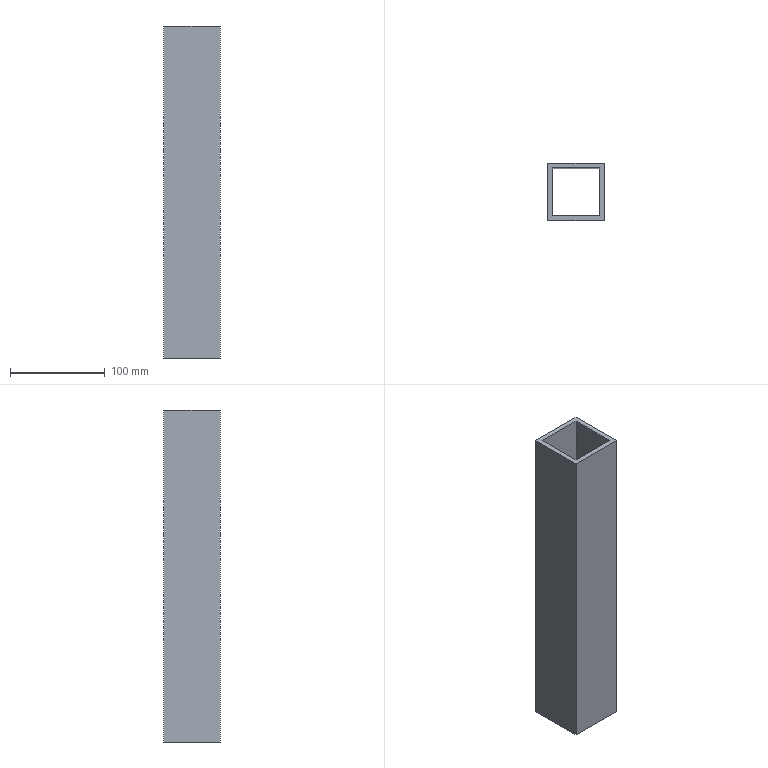Part | STEP file | Slider 12 | 1 solid | 10 faces | box 60 x 60 x 350 mm | volume 385000 mm3 | plane 10
STEP:
#1=CARTESIAN_POINT('',(-30.,30.,0.));
#2=VERTEX_POINT('',#1);
#3=CARTESIAN_POINT('',(30.,30.,0.));
#4=VERTEX_POINT('',#3);
#5=CARTESIAN_POINT('',(-30.,30.,0.));
#6=DIRECTION('',(1.,0.,0.));
#7=VECTOR('',#6,1000.);
#8=LINE('',#5,#7);
#9=EDGE_CURVE('',#2,#4,#8,.T.);
#10=ORIENTED_EDGE('',*,*,#9,.F.);
#11=CARTESIAN_POINT('',(-30.,30.,350.));
#12=VERTEX_POINT('',#11);
#13=CARTESIAN_POINT('',(-30.,30.,350.));
#14=DIRECTION('',(0.,0.,-1.));
#15=VECTOR('',#14,1000.);
#16=LINE('',#13,#15);
#17=EDGE_CURVE('',#12,#2,#16,.T.);
#18=ORIENTED_EDGE('',*,*,#17,.F.);
#19=CARTESIAN_POINT('',(30.,30.,350.));
#20=VERTEX_POINT('',#19);
#21=CARTESIAN_POINT('',(-30.,30.,350.));
#22=DIRECTION('',(1.,0.,0.));
#23=VECTOR('',#22,1000.);
#24=LINE('',#21,#23);
#25=EDGE_CURVE('',#12,#20,#24,.T.);
#26=ORIENTED_EDGE('',*,*,#25,.T.);
#27=CARTESIAN_POINT('',(30.,30.,350.));
#28=DIRECTION('',(0.,0.,-1.));
#29=VECTOR('',#28,1000.);
#30=LINE('',#27,#29);
#31=EDGE_CURVE('',#20,#4,#30,.T.);
#32=ORIENTED_EDGE('',*,*,#31,.T.);
#33=EDGE_LOOP('',(#10,#18,#26,#32));
#34=FACE_OUTER_BOUND('',#33,.T.);
#35=CARTESIAN_POINT('',(-30.,30.,350.));
#36=DIRECTION('',(0.,1.,0.));
#37=DIRECTION('',(0.,0.,1.));
#38=AXIS2_PLACEMENT_3D('',#35,#36,#37);
#39=PLANE('',#38);
#40=ADVANCED_FACE('',(#34),#39,.T.);
#41=CARTESIAN_POINT('',(-30.,-30.,0.));
#42=VERTEX_POINT('',#41);
#43=CARTESIAN_POINT('',(-30.,30.,0.));
#44=DIRECTION('',(0.,-1.,0.));
#45=VECTOR('',#44,1000.);
#46=LINE('',#43,#45);
#47=EDGE_CURVE('',#2,#42,#46,.T.);
#48=ORIENTED_EDGE('',*,*,#47,.T.);
#49=CARTESIAN_POINT('',(-30.,-30.,350.));
#50=VERTEX_POINT('',#49);
#51=CARTESIAN_POINT('',(-30.,-30.,350.));
#52=DIRECTION('',(0.,0.,-1.));
#53=VECTOR('',#52,1000.);
#54=LINE('',#51,#53);
#55=EDGE_CURVE('',#50,#42,#54,.T.);
#56=ORIENTED_EDGE('',*,*,#55,.F.);
#57=CARTESIAN_POINT('',(-30.,30.,350.));
#58=DIRECTION('',(0.,-1.,0.));
#59=VECTOR('',#58,1000.);
#60=LINE('',#57,#59);
#61=EDGE_CURVE('',#12,#50,#60,.T.);
#62=ORIENTED_EDGE('',*,*,#61,.F.);
#63=ORIENTED_EDGE('',*,*,#17,.T.);
#64=EDGE_LOOP('',(#48,#56,#62,#63));
#65=FACE_OUTER_BOUND('',#64,.T.);
#66=CARTESIAN_POINT('',(-30.,30.,350.));
#67=DIRECTION('',(1.,0.,0.));
#68=DIRECTION('',(0.,1.,0.));
#69=AXIS2_PLACEMENT_3D('',#66,#67,#68);
#70=PLANE('',#69);
#71=ADVANCED_FACE('',(#65),#70,.F.);
#72=CARTESIAN_POINT('',(30.,-30.,0.));
#73=VERTEX_POINT('',#72);
#74=CARTESIAN_POINT('',(-30.,-30.,0.));
#75=DIRECTION('',(1.,0.,0.));
#76=VECTOR('',#75,1000.);
#77=LINE('',#74,#76);
#78=EDGE_CURVE('',#42,#73,#77,.T.);
#79=ORIENTED_EDGE('',*,*,#78,.T.);
#80=CARTESIAN_POINT('',(30.,-30.,350.));
#81=VERTEX_POINT('',#80);
#82=CARTESIAN_POINT('',(30.,-30.,350.));
#83=DIRECTION('',(0.,0.,-1.));
#84=VECTOR('',#83,1000.);
#85=LINE('',#82,#84);
#86=EDGE_CURVE('',#81,#73,#85,.T.);
#87=ORIENTED_EDGE('',*,*,#86,.F.);
#88=CARTESIAN_POINT('',(-30.,-30.,350.));
#89=DIRECTION('',(1.,0.,0.));
#90=VECTOR('',#89,1000.);
#91=LINE('',#88,#90);
#92=EDGE_CURVE('',#50,#81,#91,.T.);
#93=ORIENTED_EDGE('',*,*,#92,.F.);
#94=ORIENTED_EDGE('',*,*,#55,.T.);
#95=EDGE_LOOP('',(#79,#87,#93,#94));
#96=FACE_OUTER_BOUND('',#95,.T.);
#97=CARTESIAN_POINT('',(-30.,-30.,350.));
#98=DIRECTION('',(0.,1.,0.));
#99=DIRECTION('',(0.,0.,1.));
#100=AXIS2_PLACEMENT_3D('',#97,#98,#99);
#101=PLANE('',#100);
#102=ADVANCED_FACE('',(#96),#101,.F.);
#103=CARTESIAN_POINT('',(30.,30.,0.));
#104=DIRECTION('',(0.,-1.,0.));
#105=VECTOR('',#104,1000.);
#106=LINE('',#103,#105);
#107=EDGE_CURVE('',#4,#73,#106,.T.);
#108=ORIENTED_EDGE('',*,*,#107,.F.);
#109=ORIENTED_EDGE('',*,*,#31,.F.);
#110=CARTESIAN_POINT('',(30.,30.,350.));
#111=DIRECTION('',(0.,-1.,0.));
#112=VECTOR('',#111,1000.);
#113=LINE('',#110,#112);
#114=EDGE_CURVE('',#20,#81,#113,.T.);
#115=ORIENTED_EDGE('',*,*,#114,.T.);
#116=ORIENTED_EDGE('',*,*,#86,.T.);
#117=EDGE_LOOP('',(#108,#109,#115,#116));
#118=FACE_OUTER_BOUND('',#117,.T.);
#119=CARTESIAN_POINT('',(30.,30.,350.));
#120=DIRECTION('',(1.,0.,0.));
#121=DIRECTION('',(0.,1.,0.));
#122=AXIS2_PLACEMENT_3D('',#119,#120,#121);
#123=PLANE('',#122);
#124=ADVANCED_FACE('',(#118),#123,.T.);
#125=CARTESIAN_POINT('',(-25.,25.,350.));
#126=VERTEX_POINT('',#125);
#127=CARTESIAN_POINT('',(-25.,-25.,350.));
#128=VERTEX_POINT('',#127);
#129=CARTESIAN_POINT('',(-25.,0.,350.));
#130=DIRECTION('',(0.,-1.,0.));
#131=VECTOR('',#130,1000.);
#132=LINE('',#129,#131);
#133=EDGE_CURVE('',#126,#128,#132,.T.);
#134=ORIENTED_EDGE('',*,*,#133,.F.);
#135=CARTESIAN_POINT('',(25.,25.,350.));
#136=VERTEX_POINT('',#135);
#137=CARTESIAN_POINT('',(0.,25.,350.));
#138=DIRECTION('',(1.,0.,0.));
#139=VECTOR('',#138,1000.);
#140=LINE('',#137,#139);
#141=EDGE_CURVE('',#126,#136,#140,.T.);
#142=ORIENTED_EDGE('',*,*,#141,.T.);
#143=CARTESIAN_POINT('',(25.,-25.,350.));
#144=VERTEX_POINT('',#143);
#145=CARTESIAN_POINT('',(25.,0.,350.));
#146=DIRECTION('',(0.,-1.,0.));
#147=VECTOR('',#146,1000.);
#148=LINE('',#145,#147);
#149=EDGE_CURVE('',#136,#144,#148,.T.);
#150=ORIENTED_EDGE('',*,*,#149,.T.);
#151=CARTESIAN_POINT('',(0.,-25.,350.));
#152=DIRECTION('',(1.,0.,0.));
#153=VECTOR('',#152,1000.);
#154=LINE('',#151,#153);
#155=EDGE_CURVE('',#128,#144,#154,.T.);
#156=ORIENTED_EDGE('',*,*,#155,.F.);
#157=EDGE_LOOP('',(#134,#142,#150,#156));
#158=FACE_BOUND('',#157,.T.);
#159=ORIENTED_EDGE('',*,*,#25,.F.);
#160=ORIENTED_EDGE('',*,*,#61,.T.);
#161=ORIENTED_EDGE('',*,*,#92,.T.);
#162=ORIENTED_EDGE('',*,*,#114,.F.);
#163=EDGE_LOOP('',(#159,#160,#161,#162));
#164=FACE_OUTER_BOUND('',#163,.T.);
#165=CARTESIAN_POINT('',(0.,0.,350.));
#166=DIRECTION('',(0.,0.,-1.));
#167=DIRECTION('',(-1.,0.,0.));
#168=AXIS2_PLACEMENT_3D('',#165,#166,#167);
#169=PLANE('',#168);
#170=ADVANCED_FACE('',(#158,#164),#169,.F.);
#171=CARTESIAN_POINT('',(-25.,25.,0.));
#172=VERTEX_POINT('',#171);
#173=CARTESIAN_POINT('',(25.,25.,0.));
#174=VERTEX_POINT('',#173);
#175=CARTESIAN_POINT('',(0.,25.,0.));
#176=DIRECTION('',(1.,0.,0.));
#177=VECTOR('',#176,1000.);
#178=LINE('',#175,#177);
#179=EDGE_CURVE('',#172,#174,#178,.T.);
#180=ORIENTED_EDGE('',*,*,#179,.F.);
#181=CARTESIAN_POINT('',(-25.,-25.,0.));
#182=VERTEX_POINT('',#181);
#183=CARTESIAN_POINT('',(-25.,0.,0.));
#184=DIRECTION('',(0.,-1.,0.));
#185=VECTOR('',#184,1000.);
#186=LINE('',#183,#185);
#187=EDGE_CURVE('',#172,#182,#186,.T.);
#188=ORIENTED_EDGE('',*,*,#187,.T.);
#189=CARTESIAN_POINT('',(25.,-25.,0.));
#190=VERTEX_POINT('',#189);
#191=CARTESIAN_POINT('',(0.,-25.,0.));
#192=DIRECTION('',(1.,0.,0.));
#193=VECTOR('',#192,1000.);
#194=LINE('',#191,#193);
#195=EDGE_CURVE('',#182,#190,#194,.T.);
#196=ORIENTED_EDGE('',*,*,#195,.T.);
#197=CARTESIAN_POINT('',(25.,0.,0.));
#198=DIRECTION('',(0.,-1.,0.));
#199=VECTOR('',#198,1000.);
#200=LINE('',#197,#199);
#201=EDGE_CURVE('',#174,#190,#200,.T.);
#202=ORIENTED_EDGE('',*,*,#201,.F.);
#203=EDGE_LOOP('',(#180,#188,#196,#202));
#204=FACE_BOUND('',#203,.T.);
#205=ORIENTED_EDGE('',*,*,#9,.T.);
#206=ORIENTED_EDGE('',*,*,#107,.T.);
#207=ORIENTED_EDGE('',*,*,#78,.F.);
#208=ORIENTED_EDGE('',*,*,#47,.F.);
#209=EDGE_LOOP('',(#205,#206,#207,#208));
#210=FACE_OUTER_BOUND('',#209,.T.);
#211=CARTESIAN_POINT('',(0.,0.,0.));
#212=DIRECTION('',(0.,0.,-1.));
#213=DIRECTION('',(-1.,0.,0.));
#214=AXIS2_PLACEMENT_3D('',#211,#212,#213);
#215=PLANE('',#214);
#216=ADVANCED_FACE('',(#204,#210),#215,.T.);
#217=ORIENTED_EDGE('',*,*,#179,.T.);
#218=CARTESIAN_POINT('',(25.,25.,350.));
#219=DIRECTION('',(0.,0.,-1.));
#220=VECTOR('',#219,1000.);
#221=LINE('',#218,#220);
#222=EDGE_CURVE('',#136,#174,#221,.T.);
#223=ORIENTED_EDGE('',*,*,#222,.F.);
#224=ORIENTED_EDGE('',*,*,#141,.F.);
#225=CARTESIAN_POINT('',(-25.,25.,350.));
#226=DIRECTION('',(0.,0.,-1.));
#227=VECTOR('',#226,1000.);
#228=LINE('',#225,#227);
#229=EDGE_CURVE('',#126,#172,#228,.T.);
#230=ORIENTED_EDGE('',*,*,#229,.T.);
#231=EDGE_LOOP('',(#217,#223,#224,#230));
#232=FACE_OUTER_BOUND('',#231,.T.);
#233=CARTESIAN_POINT('',(0.,25.,350.));
#234=DIRECTION('',(0.,1.,0.));
#235=DIRECTION('',(0.,0.,1.));
#236=AXIS2_PLACEMENT_3D('',#233,#234,#235);
#237=PLANE('',#236);
#238=ADVANCED_FACE('',(#232),#237,.F.);
#239=ORIENTED_EDGE('',*,*,#187,.F.);
#240=ORIENTED_EDGE('',*,*,#229,.F.);
#241=ORIENTED_EDGE('',*,*,#133,.T.);
#242=CARTESIAN_POINT('',(-25.,-25.,350.));
#243=DIRECTION('',(0.,0.,-1.));
#244=VECTOR('',#243,1000.);
#245=LINE('',#242,#244);
#246=EDGE_CURVE('',#128,#182,#245,.T.);
#247=ORIENTED_EDGE('',*,*,#246,.T.);
#248=EDGE_LOOP('',(#239,#240,#241,#247));
#249=FACE_OUTER_BOUND('',#248,.T.);
#250=CARTESIAN_POINT('',(-25.,0.,350.));
#251=DIRECTION('',(1.,0.,0.));
#252=DIRECTION('',(0.,1.,0.));
#253=AXIS2_PLACEMENT_3D('',#250,#251,#252);
#254=PLANE('',#253);
#255=ADVANCED_FACE('',(#249),#254,.T.);
#256=ORIENTED_EDGE('',*,*,#195,.F.);
#257=ORIENTED_EDGE('',*,*,#246,.F.);
#258=ORIENTED_EDGE('',*,*,#155,.T.);
#259=CARTESIAN_POINT('',(25.,-25.,350.));
#260=DIRECTION('',(0.,0.,-1.));
#261=VECTOR('',#260,1000.);
#262=LINE('',#259,#261);
#263=EDGE_CURVE('',#144,#190,#262,.T.);
#264=ORIENTED_EDGE('',*,*,#263,.T.);
#265=EDGE_LOOP('',(#256,#257,#258,#264));
#266=FACE_OUTER_BOUND('',#265,.T.);
#267=CARTESIAN_POINT('',(0.,-25.,350.));
#268=DIRECTION('',(0.,1.,0.));
#269=DIRECTION('',(0.,0.,1.));
#270=AXIS2_PLACEMENT_3D('',#267,#268,#269);
#271=PLANE('',#270);
#272=ADVANCED_FACE('',(#266),#271,.T.);
#273=ORIENTED_EDGE('',*,*,#201,.T.);
#274=ORIENTED_EDGE('',*,*,#263,.F.);
#275=ORIENTED_EDGE('',*,*,#149,.F.);
#276=ORIENTED_EDGE('',*,*,#222,.T.);
#277=EDGE_LOOP('',(#273,#274,#275,#276));
#278=FACE_OUTER_BOUND('',#277,.T.);
#279=CARTESIAN_POINT('',(25.,0.,350.));
#280=DIRECTION('',(1.,0.,0.));
#281=DIRECTION('',(0.,1.,0.));
#282=AXIS2_PLACEMENT_3D('',#279,#280,#281);
#283=PLANE('',#282);
#284=ADVANCED_FACE('',(#278),#283,.F.);
#285=CLOSED_SHELL('',(#40,#71,#102,#124,#170,#216,#238,#255,#272,#284));
#286=MANIFOLD_SOLID_BREP('',#285);
#287=CARTESIAN_POINT('',(0.,0.,0.));
#288=DIRECTION('',(0.,0.,1.));
#289=DIRECTION('',(1.,0.,0.));
#290=AXIS2_PLACEMENT_3D('',#287,#288,#289);
#291=(LENGTH_UNIT()NAMED_UNIT(*)SI_UNIT(.MILLI.,.METRE.));
#292=UNCERTAINTY_MEASURE_WITH_UNIT(LENGTH_MEASURE(0.00001),#291,'','');
#293=(NAMED_UNIT(*)PLANE_ANGLE_UNIT()SI_UNIT($,.RADIAN.));
#294=(NAMED_UNIT(*)SI_UNIT($,.STERADIAN.)SOLID_ANGLE_UNIT());
#295=(GEOMETRIC_REPRESENTATION_CONTEXT(3)GLOBAL_UNCERTAINTY_ASSIGNED_CONTEXT((#292))GLOBAL_UNIT_ASSIGNED_CONTEXT((#291,#293,#294))REPRESENTATION_CONTEXT('',''));
#296=ADVANCED_BREP_SHAPE_REPRESENTATION('',(#286,#290),#295);